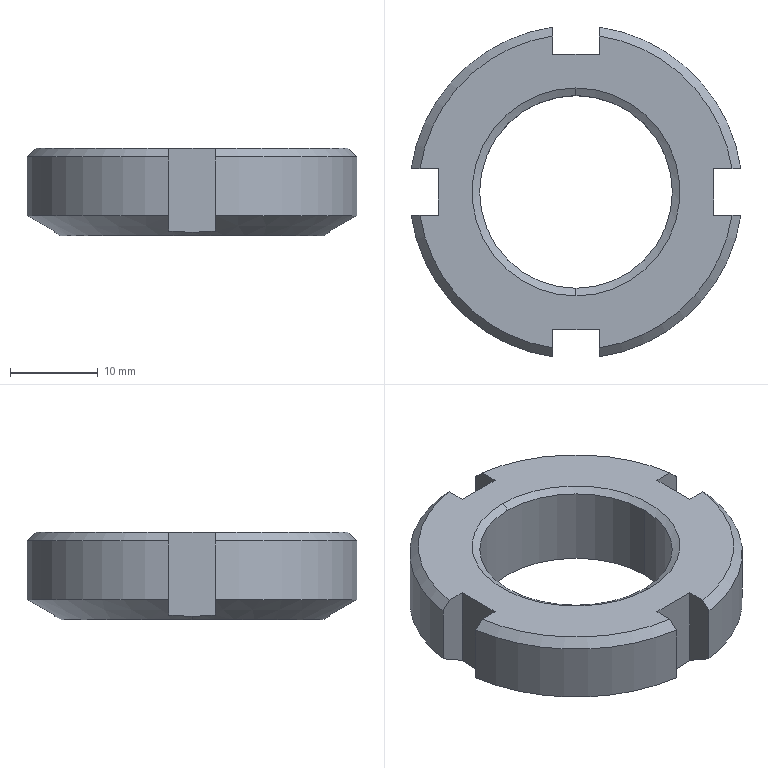Part | SolidWorks | features BaseBody 1 | 1 solid | 30 faces | box 37.629 x 37.629 x 10 mm | volume 6359 mm3 | plane 14 | cone 10 | cylinder 6 | commonest cylinder face diameters 38 x4 22 x2
STEP:
#1=CARTESIAN_POINT('',(0.,11.,9.5));
#2=VERTEX_POINT('',#1);
#3=CARTESIAN_POINT('',(-11.,0.,9.5));
#4=VERTEX_POINT('',#3);
#5=CARTESIAN_POINT('',(0.,0.,9.5));
#6=DIRECTION('',(0.,0.,1.));
#7=DIRECTION('',(1.,0.,0.));
#8=AXIS2_PLACEMENT_3D('',#5,#6,#7);
#9=CIRCLE('',#8,11.);
#10=EDGE_CURVE('',#2,#4,#9,.T.);
#11=ORIENTED_EDGE('',*,*,#10,.F.);
#12=CARTESIAN_POINT('',(0.,11.866,10.));
#13=VERTEX_POINT('',#12);
#14=CARTESIAN_POINT('',(0.,11.866,10.));
#15=DIRECTION('',(0.,0.866,0.5));
#16=VECTOR('',#15,1000.);
#17=LINE('',#14,#16);
#18=EDGE_CURVE('',#2,#13,#17,.T.);
#19=ORIENTED_EDGE('',*,*,#18,.T.);
#20=CARTESIAN_POINT('',(0.,-11.866,10.));
#21=VERTEX_POINT('',#20);
#22=CARTESIAN_POINT('',(0.,0.,10.));
#23=DIRECTION('',(0.,0.,-1.));
#24=DIRECTION('',(0.,-1.,0.));
#25=AXIS2_PLACEMENT_3D('',#22,#23,#24);
#26=CIRCLE('',#25,11.866);
#27=EDGE_CURVE('',#21,#13,#26,.T.);
#28=ORIENTED_EDGE('',*,*,#27,.F.);
#29=CARTESIAN_POINT('',(0.,-11.,9.5));
#30=VERTEX_POINT('',#29);
#31=CARTESIAN_POINT('',(0.,-11.866,10.));
#32=DIRECTION('',(0.,-0.866,0.5));
#33=VECTOR('',#32,1000.);
#34=LINE('',#31,#33);
#35=EDGE_CURVE('',#30,#21,#34,.T.);
#36=ORIENTED_EDGE('',*,*,#35,.F.);
#37=CARTESIAN_POINT('',(0.,0.,9.5));
#38=DIRECTION('',(0.,0.,1.));
#39=DIRECTION('',(1.,0.,0.));
#40=AXIS2_PLACEMENT_3D('',#37,#38,#39);
#41=CIRCLE('',#40,11.);
#42=EDGE_CURVE('',#4,#30,#41,.T.);
#43=ORIENTED_EDGE('',*,*,#42,.F.);
#44=EDGE_LOOP('',(#11,#19,#28,#36,#43));
#45=FACE_OUTER_BOUND('',#44,.T.);
#46=CARTESIAN_POINT('',(0.,0.,10.));
#47=DIRECTION('',(0.,0.,1.));
#48=DIRECTION('',(0.,-1.,0.));
#49=AXIS2_PLACEMENT_3D('',#46,#47,#48);
#50=CONICAL_SURFACE('',#49,11.866,1.047);
#51=ADVANCED_FACE('',(#45),#50,.F.);
#52=CARTESIAN_POINT('',(15.,0.,0.));
#53=VERTEX_POINT('',#52);
#54=CARTESIAN_POINT('',(-15.,0.,0.));
#55=VERTEX_POINT('',#54);
#56=CARTESIAN_POINT('',(0.,0.,0.));
#57=DIRECTION('',(0.,0.,1.));
#58=DIRECTION('',(1.,0.,0.));
#59=AXIS2_PLACEMENT_3D('',#56,#57,#58);
#60=CIRCLE('',#59,15.);
#61=EDGE_CURVE('',#53,#55,#60,.T.);
#62=ORIENTED_EDGE('',*,*,#61,.T.);
#63=CARTESIAN_POINT('',(-15.714,0.,0.4124));
#64=VERTEX_POINT('',#63);
#65=CARTESIAN_POINT('',(-19.,0.,2.309));
#66=DIRECTION('',(-0.866,0.,0.5));
#67=VECTOR('',#66,1000.);
#68=LINE('',#65,#67);
#69=EDGE_CURVE('',#55,#64,#68,.T.);
#70=ORIENTED_EDGE('',*,*,#69,.T.);
#71=CARTESIAN_POINT('',(-15.714,2.65,0.5405));
#72=VERTEX_POINT('',#71);
#73=CARTESIAN_POINT('',(-15.714,0.,0.4124));
#74=CARTESIAN_POINT('',(-15.714,0.8854,0.4124));
#75=CARTESIAN_POINT('',(-15.714,1.769,0.4559));
#76=CARTESIAN_POINT('',(-15.714,2.65,0.5405));
#77=B_SPLINE_CURVE_WITH_KNOTS('',3,(#73,#74,#75,#76),.UNSPECIFIED.,.F.,.F.,(4,4),(0.,0.002653),.UNSPECIFIED.);
#78=EDGE_CURVE('',#64,#72,#77,.T.);
#79=ORIENTED_EDGE('',*,*,#78,.T.);
#80=CARTESIAN_POINT('',(-18.814,2.65,2.309));
#81=VERTEX_POINT('',#80);
#82=CARTESIAN_POINT('',(-15.714,2.65,0.5405));
#83=CARTESIAN_POINT('',(-16.748,2.65,1.129));
#84=CARTESIAN_POINT('',(-17.781,2.65,1.719));
#85=CARTESIAN_POINT('',(-18.814,2.65,2.309));
#86=B_SPLINE_CURVE_WITH_KNOTS('',3,(#82,#83,#84,#85),.UNSPECIFIED.,.F.,.F.,(4,4),(0.,0.003569),.UNSPECIFIED.);
#87=EDGE_CURVE('',#72,#81,#86,.T.);
#88=ORIENTED_EDGE('',*,*,#87,.T.);
#89=CARTESIAN_POINT('',(-2.65,18.814,2.309));
#90=VERTEX_POINT('',#89);
#91=CARTESIAN_POINT('',(0.,0.,2.309));
#92=DIRECTION('',(0.,0.,-1.));
#93=DIRECTION('',(1.,0.,0.));
#94=AXIS2_PLACEMENT_3D('',#91,#92,#93);
#95=CIRCLE('',#94,19.);
#96=EDGE_CURVE('',#81,#90,#95,.T.);
#97=ORIENTED_EDGE('',*,*,#96,.T.);
#98=CARTESIAN_POINT('',(-2.65,15.714,0.5405));
#99=VERTEX_POINT('',#98);
#100=CARTESIAN_POINT('',(-2.65,18.814,2.309));
#101=CARTESIAN_POINT('',(-2.65,17.781,1.719));
#102=CARTESIAN_POINT('',(-2.65,16.748,1.129));
#103=CARTESIAN_POINT('',(-2.65,15.714,0.5405));
#104=B_SPLINE_CURVE_WITH_KNOTS('',3,(#100,#101,#102,#103),.UNSPECIFIED.,.F.,.F.,(4,4),(0.,0.003569),.UNSPECIFIED.);
#105=EDGE_CURVE('',#90,#99,#104,.T.);
#106=ORIENTED_EDGE('',*,*,#105,.T.);
#107=CARTESIAN_POINT('',(2.65,15.714,0.5405));
#108=VERTEX_POINT('',#107);
#109=CARTESIAN_POINT('',(-2.65,15.714,0.5405));
#110=CARTESIAN_POINT('',(-0.8833,15.714,0.3709));
#111=CARTESIAN_POINT('',(0.8833,15.714,0.3709));
#112=CARTESIAN_POINT('',(2.65,15.714,0.5405));
#113=B_SPLINE_CURVE_WITH_KNOTS('',3,(#109,#110,#111,#112),.UNSPECIFIED.,.F.,.F.,(4,4),(0.,0.0053),.UNSPECIFIED.);
#114=EDGE_CURVE('',#99,#108,#113,.T.);
#115=ORIENTED_EDGE('',*,*,#114,.T.);
#116=CARTESIAN_POINT('',(2.65,18.814,2.309));
#117=VERTEX_POINT('',#116);
#118=CARTESIAN_POINT('',(2.65,15.714,0.5405));
#119=CARTESIAN_POINT('',(2.65,16.748,1.129));
#120=CARTESIAN_POINT('',(2.65,17.781,1.719));
#121=CARTESIAN_POINT('',(2.65,18.814,2.309));
#122=B_SPLINE_CURVE_WITH_KNOTS('',3,(#118,#119,#120,#121),.UNSPECIFIED.,.F.,.F.,(4,4),(0.,0.003569),.UNSPECIFIED.);
#123=EDGE_CURVE('',#108,#117,#122,.T.);
#124=ORIENTED_EDGE('',*,*,#123,.T.);
#125=CARTESIAN_POINT('',(18.814,2.65,2.309));
#126=VERTEX_POINT('',#125);
#127=CARTESIAN_POINT('',(0.,0.,2.309));
#128=DIRECTION('',(0.,0.,-1.));
#129=DIRECTION('',(1.,0.,0.));
#130=AXIS2_PLACEMENT_3D('',#127,#128,#129);
#131=CIRCLE('',#130,19.);
#132=EDGE_CURVE('',#117,#126,#131,.T.);
#133=ORIENTED_EDGE('',*,*,#132,.T.);
#134=CARTESIAN_POINT('',(15.714,2.65,0.5405));
#135=VERTEX_POINT('',#134);
#136=CARTESIAN_POINT('',(18.814,2.65,2.309));
#137=CARTESIAN_POINT('',(17.781,2.65,1.719));
#138=CARTESIAN_POINT('',(16.748,2.65,1.129));
#139=CARTESIAN_POINT('',(15.714,2.65,0.5405));
#140=B_SPLINE_CURVE_WITH_KNOTS('',3,(#136,#137,#138,#139),.UNSPECIFIED.,.F.,.F.,(4,4),(0.,0.003569),.UNSPECIFIED.);
#141=EDGE_CURVE('',#126,#135,#140,.T.);
#142=ORIENTED_EDGE('',*,*,#141,.T.);
#143=CARTESIAN_POINT('',(15.714,0.,0.4124));
#144=VERTEX_POINT('',#143);
#145=CARTESIAN_POINT('',(15.714,2.65,0.5405));
#146=CARTESIAN_POINT('',(15.714,1.769,0.4559));
#147=CARTESIAN_POINT('',(15.714,0.8854,0.4124));
#148=CARTESIAN_POINT('',(15.714,0.,0.4124));
#149=B_SPLINE_CURVE_WITH_KNOTS('',3,(#145,#146,#147,#148),.UNSPECIFIED.,.F.,.F.,(4,4),(-0.002653,0.),.UNSPECIFIED.);
#150=EDGE_CURVE('',#135,#144,#149,.T.);
#151=ORIENTED_EDGE('',*,*,#150,.T.);
#152=CARTESIAN_POINT('',(19.,0.,2.309));
#153=DIRECTION('',(0.866,0.,0.5));
#154=VECTOR('',#153,1000.);
#155=LINE('',#152,#154);
#156=EDGE_CURVE('',#53,#144,#155,.T.);
#157=ORIENTED_EDGE('',*,*,#156,.F.);
#158=EDGE_LOOP('',(#62,#70,#79,#88,#97,#106,#115,#124,#133,#142,#151,#157));
#159=FACE_OUTER_BOUND('',#158,.T.);
#160=CARTESIAN_POINT('',(0.,0.,2.309));
#161=DIRECTION('',(0.,0.,1.));
#162=DIRECTION('',(1.,0.,0.));
#163=AXIS2_PLACEMENT_3D('',#160,#161,#162);
#164=CONICAL_SURFACE('',#163,19.,1.047);
#165=ADVANCED_FACE('',(#159),#164,.T.);
#166=ORIENTED_EDGE('',*,*,#42,.T.);
#167=CARTESIAN_POINT('',(11.,0.,9.5));
#168=VERTEX_POINT('',#167);
#169=CARTESIAN_POINT('',(0.,0.,9.5));
#170=DIRECTION('',(0.,0.,1.));
#171=DIRECTION('',(1.,0.,0.));
#172=AXIS2_PLACEMENT_3D('',#169,#170,#171);
#173=CIRCLE('',#172,11.);
#174=EDGE_CURVE('',#30,#168,#173,.T.);
#175=ORIENTED_EDGE('',*,*,#174,.T.);
#176=CARTESIAN_POINT('',(11.,0.,0.5));
#177=VERTEX_POINT('',#176);
#178=CARTESIAN_POINT('',(11.,0.,10.));
#179=DIRECTION('',(0.,0.,-1.));
#180=VECTOR('',#179,1000.);
#181=LINE('',#178,#180);
#182=EDGE_CURVE('',#168,#177,#181,.T.);
#183=ORIENTED_EDGE('',*,*,#182,.T.);
#184=CARTESIAN_POINT('',(-11.,0.,0.5));
#185=VERTEX_POINT('',#184);
#186=CARTESIAN_POINT('',(0.,0.,0.5));
#187=DIRECTION('',(0.,0.,1.));
#188=DIRECTION('',(-1.,0.,0.));
#189=AXIS2_PLACEMENT_3D('',#186,#187,#188);
#190=CIRCLE('',#189,11.);
#191=EDGE_CURVE('',#185,#177,#190,.T.);
#192=ORIENTED_EDGE('',*,*,#191,.F.);
#193=CARTESIAN_POINT('',(-11.,0.,10.));
#194=DIRECTION('',(0.,0.,-1.));
#195=VECTOR('',#194,1000.);
#196=LINE('',#193,#195);
#197=EDGE_CURVE('',#4,#185,#196,.T.);
#198=ORIENTED_EDGE('',*,*,#197,.F.);
#199=EDGE_LOOP('',(#166,#175,#183,#192,#198));
#200=FACE_OUTER_BOUND('',#199,.T.);
#201=CARTESIAN_POINT('',(0.,0.,10.));
#202=DIRECTION('',(0.,0.,-1.));
#203=DIRECTION('',(-1.,0.,0.));
#204=AXIS2_PLACEMENT_3D('',#201,#202,#203);
#205=CYLINDRICAL_SURFACE('',#204,11.);
#206=ADVANCED_FACE('',(#200),#205,.F.);
#207=ORIENTED_EDGE('',*,*,#191,.T.);
#208=CARTESIAN_POINT('',(11.866,0.,0.));
#209=VERTEX_POINT('',#208);
#210=CARTESIAN_POINT('',(11.866,0.,0.));
#211=DIRECTION('',(0.866,0.,-0.5));
#212=VECTOR('',#211,1000.);
#213=LINE('',#210,#212);
#214=EDGE_CURVE('',#177,#209,#213,.T.);
#215=ORIENTED_EDGE('',*,*,#214,.T.);
#216=CARTESIAN_POINT('',(-11.866,0.,0.));
#217=VERTEX_POINT('',#216);
#218=CARTESIAN_POINT('',(0.,0.,0.));
#219=DIRECTION('',(0.,0.,-1.));
#220=DIRECTION('',(-1.,0.,0.));
#221=AXIS2_PLACEMENT_3D('',#218,#219,#220);
#222=CIRCLE('',#221,11.866);
#223=EDGE_CURVE('',#209,#217,#222,.T.);
#224=ORIENTED_EDGE('',*,*,#223,.T.);
#225=CARTESIAN_POINT('',(-11.866,0.,0.));
#226=DIRECTION('',(-0.866,0.,-0.5));
#227=VECTOR('',#226,1000.);
#228=LINE('',#225,#227);
#229=EDGE_CURVE('',#185,#217,#228,.T.);
#230=ORIENTED_EDGE('',*,*,#229,.F.);
#231=EDGE_LOOP('',(#207,#215,#224,#230));
#232=FACE_OUTER_BOUND('',#231,.T.);
#233=CARTESIAN_POINT('',(0.,0.,0.));
#234=DIRECTION('',(0.,0.,-1.));
#235=DIRECTION('',(-1.,0.,0.));
#236=AXIS2_PLACEMENT_3D('',#233,#234,#235);
#237=CONICAL_SURFACE('',#236,11.866,1.047);
#238=ADVANCED_FACE('',(#232),#237,.F.);
#239=CARTESIAN_POINT('',(17.804,-2.65,10.));
#240=VERTEX_POINT('',#239);
#241=CARTESIAN_POINT('',(15.714,-2.65,10.));
#242=VERTEX_POINT('',#241);
#243=CARTESIAN_POINT('',(0.,-2.65,10.));
#244=DIRECTION('',(-1.,0.,0.));
#245=VECTOR('',#244,1000.);
#246=LINE('',#243,#245);
#247=EDGE_CURVE('',#240,#242,#246,.T.);
#248=ORIENTED_EDGE('',*,*,#247,.T.);
#249=CARTESIAN_POINT('',(15.714,2.65,10.));
#250=VERTEX_POINT('',#249);
#251=CARTESIAN_POINT('',(15.714,0.,10.));
#252=DIRECTION('',(0.,1.,0.));
#253=VECTOR('',#252,1000.);
#254=LINE('',#251,#253);
#255=EDGE_CURVE('',#242,#250,#254,.T.);
#256=ORIENTED_EDGE('',*,*,#255,.T.);
#257=CARTESIAN_POINT('',(17.804,2.65,10.));
#258=VERTEX_POINT('',#257);
#259=CARTESIAN_POINT('',(0.,2.65,10.));
#260=DIRECTION('',(1.,0.,0.));
#261=VECTOR('',#260,1000.);
#262=LINE('',#259,#261);
#263=EDGE_CURVE('',#250,#258,#262,.T.);
#264=ORIENTED_EDGE('',*,*,#263,.T.);
#265=CARTESIAN_POINT('',(2.65,17.804,10.));
#266=VERTEX_POINT('',#265);
#267=CARTESIAN_POINT('',(0.,0.,10.));
#268=DIRECTION('',(0.,0.,1.));
#269=DIRECTION('',(-1.,0.,0.));
#270=AXIS2_PLACEMENT_3D('',#267,#268,#269);
#271=CIRCLE('',#270,18.);
#272=EDGE_CURVE('',#258,#266,#271,.T.);
#273=ORIENTED_EDGE('',*,*,#272,.T.);
#274=CARTESIAN_POINT('',(2.65,15.714,10.));
#275=VERTEX_POINT('',#274);
#276=CARTESIAN_POINT('',(2.65,0.,10.));
#277=DIRECTION('',(0.,-1.,0.));
#278=VECTOR('',#277,1000.);
#279=LINE('',#276,#278);
#280=EDGE_CURVE('',#266,#275,#279,.T.);
#281=ORIENTED_EDGE('',*,*,#280,.T.);
#282=CARTESIAN_POINT('',(-2.65,15.714,10.));
#283=VERTEX_POINT('',#282);
#284=CARTESIAN_POINT('',(0.,15.714,10.));
#285=DIRECTION('',(-1.,0.,0.));
#286=VECTOR('',#285,1000.);
#287=LINE('',#284,#286);
#288=EDGE_CURVE('',#275,#283,#287,.T.);
#289=ORIENTED_EDGE('',*,*,#288,.T.);
#290=CARTESIAN_POINT('',(-2.65,17.804,10.));
#291=VERTEX_POINT('',#290);
#292=CARTESIAN_POINT('',(-2.65,0.,10.));
#293=DIRECTION('',(0.,1.,0.));
#294=VECTOR('',#293,1000.);
#295=LINE('',#292,#294);
#296=EDGE_CURVE('',#283,#291,#295,.T.);
#297=ORIENTED_EDGE('',*,*,#296,.T.);
#298=CARTESIAN_POINT('',(-17.804,2.65,10.));
#299=VERTEX_POINT('',#298);
#300=CARTESIAN_POINT('',(0.,0.,10.));
#301=DIRECTION('',(0.,0.,1.));
#302=DIRECTION('',(0.,1.,0.));
#303=AXIS2_PLACEMENT_3D('',#300,#301,#302);
#304=CIRCLE('',#303,18.);
#305=EDGE_CURVE('',#291,#299,#304,.T.);
#306=ORIENTED_EDGE('',*,*,#305,.T.);
#307=CARTESIAN_POINT('',(-15.714,2.65,10.));
#308=VERTEX_POINT('',#307);
#309=CARTESIAN_POINT('',(0.,2.65,10.));
#310=DIRECTION('',(1.,0.,0.));
#311=VECTOR('',#310,1000.);
#312=LINE('',#309,#311);
#313=EDGE_CURVE('',#299,#308,#312,.T.);
#314=ORIENTED_EDGE('',*,*,#313,.T.);
#315=CARTESIAN_POINT('',(-15.714,-2.65,10.));
#316=VERTEX_POINT('',#315);
#317=CARTESIAN_POINT('',(-15.714,0.,10.));
#318=DIRECTION('',(0.,-1.,0.));
#319=VECTOR('',#318,1000.);
#320=LINE('',#317,#319);
#321=EDGE_CURVE('',#308,#316,#320,.T.);
#322=ORIENTED_EDGE('',*,*,#321,.T.);
#323=CARTESIAN_POINT('',(-17.804,-2.65,10.));
#324=VERTEX_POINT('',#323);
#325=CARTESIAN_POINT('',(0.,-2.65,10.));
#326=DIRECTION('',(-1.,0.,0.));
#327=VECTOR('',#326,1000.);
#328=LINE('',#325,#327);
#329=EDGE_CURVE('',#316,#324,#328,.T.);
#330=ORIENTED_EDGE('',*,*,#329,.T.);
#331=CARTESIAN_POINT('',(-2.65,-17.804,10.));
#332=VERTEX_POINT('',#331);
#333=CARTESIAN_POINT('',(0.,0.,10.));
#334=DIRECTION('',(0.,0.,1.));
#335=DIRECTION('',(-1.,0.,0.));
#336=AXIS2_PLACEMENT_3D('',#333,#334,#335);
#337=CIRCLE('',#336,18.);
#338=EDGE_CURVE('',#324,#332,#337,.T.);
#339=ORIENTED_EDGE('',*,*,#338,.T.);
#340=CARTESIAN_POINT('',(-2.65,-15.714,10.));
#341=VERTEX_POINT('',#340);
#342=CARTESIAN_POINT('',(-2.65,0.,10.));
#343=DIRECTION('',(0.,1.,0.));
#344=VECTOR('',#343,1000.);
#345=LINE('',#342,#344);
#346=EDGE_CURVE('',#332,#341,#345,.T.);
#347=ORIENTED_EDGE('',*,*,#346,.T.);
#348=CARTESIAN_POINT('',(2.65,-15.714,10.));
#349=VERTEX_POINT('',#348);
#350=CARTESIAN_POINT('',(0.,-15.714,10.));
#351=DIRECTION('',(1.,0.,0.));
#352=VECTOR('',#351,1000.);
#353=LINE('',#350,#352);
#354=EDGE_CURVE('',#341,#349,#353,.T.);
#355=ORIENTED_EDGE('',*,*,#354,.T.);
#356=CARTESIAN_POINT('',(2.65,-17.804,10.));
#357=VERTEX_POINT('',#356);
#358=CARTESIAN_POINT('',(2.65,0.,10.));
#359=DIRECTION('',(0.,-1.,0.));
#360=VECTOR('',#359,1000.);
#361=LINE('',#358,#360);
#362=EDGE_CURVE('',#349,#357,#361,.T.);
#363=ORIENTED_EDGE('',*,*,#362,.T.);
#364=CARTESIAN_POINT('',(0.,0.,10.));
#365=DIRECTION('',(0.,0.,1.));
#366=DIRECTION('',(-1.,0.,0.));
#367=AXIS2_PLACEMENT_3D('',#364,#365,#366);
#368=CIRCLE('',#367,18.);
#369=EDGE_CURVE('',#357,#240,#368,.T.);
#370=ORIENTED_EDGE('',*,*,#369,.T.);
#371=EDGE_LOOP('',(#248,#256,#264,#273,#281,#289,#297,#306,#314,#322,#330,#339,#347,#355,#363,#370));
#372=FACE_OUTER_BOUND('',#371,.T.);
#373=ORIENTED_EDGE('',*,*,#27,.T.);
#374=CARTESIAN_POINT('',(0.,0.,10.));
#375=DIRECTION('',(0.,0.,-1.));
#376=DIRECTION('',(0.,-1.,0.));
#377=AXIS2_PLACEMENT_3D('',#374,#375,#376);
#378=CIRCLE('',#377,11.866);
#379=EDGE_CURVE('',#13,#21,#378,.T.);
#380=ORIENTED_EDGE('',*,*,#379,.T.);
#381=EDGE_LOOP('',(#373,#380));
#382=FACE_BOUND('',#381,.T.);
#383=CARTESIAN_POINT('',(0.,0.,10.));
#384=DIRECTION('',(0.,0.,1.));
#385=DIRECTION('',(1.,0.,0.));
#386=AXIS2_PLACEMENT_3D('',#383,#384,#385);
#387=PLANE('',#386);
#388=ADVANCED_FACE('',(#372,#382),#387,.T.);
#389=ORIENTED_EDGE('',*,*,#150,.F.);
#390=CARTESIAN_POINT('',(15.714,2.65,0.));
#391=DIRECTION('',(0.,0.,-1.));
#392=VECTOR('',#391,1000.);
#393=LINE('',#390,#392);
#394=EDGE_CURVE('',#250,#135,#393,.T.);
#395=ORIENTED_EDGE('',*,*,#394,.F.);
#396=ORIENTED_EDGE('',*,*,#255,.F.);
#397=CARTESIAN_POINT('',(15.714,-2.65,0.5405));
#398=VERTEX_POINT('',#397);
#399=CARTESIAN_POINT('',(15.714,-2.65,0.));
#400=DIRECTION('',(0.,0.,1.));
#401=VECTOR('',#400,1000.);
#402=LINE('',#399,#401);
#403=EDGE_CURVE('',#398,#242,#402,.T.);
#404=ORIENTED_EDGE('',*,*,#403,.F.);
#405=CARTESIAN_POINT('',(15.714,0.,0.4124));
#406=CARTESIAN_POINT('',(15.714,-0.8854,0.4124));
#407=CARTESIAN_POINT('',(15.714,-1.769,0.4559));
#408=CARTESIAN_POINT('',(15.714,-2.65,0.5405));
#409=B_SPLINE_CURVE_WITH_KNOTS('',3,(#405,#406,#407,#408),.UNSPECIFIED.,.F.,.F.,(4,4),(0.,0.002653),.UNSPECIFIED.);
#410=EDGE_CURVE('',#144,#398,#409,.T.);
#411=ORIENTED_EDGE('',*,*,#410,.F.);
#412=EDGE_LOOP('',(#389,#395,#396,#404,#411));
#413=FACE_OUTER_BOUND('',#412,.T.);
#414=CARTESIAN_POINT('',(15.714,-2.65,0.));
#415=DIRECTION('',(-1.,0.,0.));
#416=DIRECTION('',(0.,-1.,0.));
#417=AXIS2_PLACEMENT_3D('',#414,#415,#416);
#418=PLANE('',#417);
#419=ADVANCED_FACE('',(#413),#418,.F.);
#420=CARTESIAN_POINT('',(18.814,-2.65,2.309));
#421=VERTEX_POINT('',#420);
#422=CARTESIAN_POINT('',(18.814,-2.65,9.));
#423=VERTEX_POINT('',#422);
#424=CARTESIAN_POINT('',(18.814,-2.65,0.));
#425=DIRECTION('',(0.,0.,1.));
#426=VECTOR('',#425,1000.);
#427=LINE('',#424,#426);
#428=EDGE_CURVE('',#421,#423,#427,.T.);
#429=ORIENTED_EDGE('',*,*,#428,.F.);
#430=CARTESIAN_POINT('',(15.714,-2.65,0.5405));
#431=CARTESIAN_POINT('',(16.748,-2.65,1.129));
#432=CARTESIAN_POINT('',(17.781,-2.65,1.719));
#433=CARTESIAN_POINT('',(18.814,-2.65,2.309));
#434=B_SPLINE_CURVE_WITH_KNOTS('',3,(#430,#431,#432,#433),.UNSPECIFIED.,.F.,.F.,(4,4),(0.,0.003569),.UNSPECIFIED.);
#435=EDGE_CURVE('',#398,#421,#434,.T.);
#436=ORIENTED_EDGE('',*,*,#435,.F.);
#437=ORIENTED_EDGE('',*,*,#403,.T.);
#438=ORIENTED_EDGE('',*,*,#247,.F.);
#439=CARTESIAN_POINT('',(18.814,-2.65,9.));
#440=CARTESIAN_POINT('',(18.478,-2.65,9.333));
#441=CARTESIAN_POINT('',(18.141,-2.65,9.667));
#442=CARTESIAN_POINT('',(17.804,-2.65,10.));
#443=B_SPLINE_CURVE_WITH_KNOTS('',3,(#439,#440,#441,#442),.UNSPECIFIED.,.F.,.F.,(4,4),(0.,0.001422),.UNSPECIFIED.);
#444=EDGE_CURVE('',#423,#240,#443,.T.);
#445=ORIENTED_EDGE('',*,*,#444,.F.);
#446=EDGE_LOOP('',(#429,#436,#437,#438,#445));
#447=FACE_OUTER_BOUND('',#446,.T.);
#448=CARTESIAN_POINT('',(15.714,-2.65,0.));
#449=DIRECTION('',(0.,-1.,0.));
#450=DIRECTION('',(1.,0.,0.));
#451=AXIS2_PLACEMENT_3D('',#448,#449,#450);
#452=PLANE('',#451);
#453=ADVANCED_FACE('',(#447),#452,.F.);
#454=CARTESIAN_POINT('',(2.65,-18.814,9.));
#455=VERTEX_POINT('',#454);
#456=CARTESIAN_POINT('',(2.65,-17.804,10.));
#457=CARTESIAN_POINT('',(2.65,-18.141,9.667));
#458=CARTESIAN_POINT('',(2.65,-18.478,9.333));
#459=CARTESIAN_POINT('',(2.65,-18.814,9.));
#460=B_SPLINE_CURVE_WITH_KNOTS('',3,(#456,#457,#458,#459),.UNSPECIFIED.,.F.,.F.,(4,4),(0.,0.001422),.UNSPECIFIED.);
#461=EDGE_CURVE('',#357,#455,#460,.T.);
#462=ORIENTED_EDGE('',*,*,#461,.T.);
#463=CARTESIAN_POINT('',(0.,0.,9.));
#464=DIRECTION('',(0.,0.,1.));
#465=DIRECTION('',(-1.,0.,0.));
#466=AXIS2_PLACEMENT_3D('',#463,#464,#465);
#467=CIRCLE('',#466,19.);
#468=EDGE_CURVE('',#455,#423,#467,.T.);
#469=ORIENTED_EDGE('',*,*,#468,.T.);
#470=ORIENTED_EDGE('',*,*,#444,.T.);
#471=ORIENTED_EDGE('',*,*,#369,.F.);
#472=EDGE_LOOP('',(#462,#469,#470,#471));
#473=FACE_OUTER_BOUND('',#472,.T.);
#474=CARTESIAN_POINT('',(0.,0.,9.));
#475=DIRECTION('',(0.,0.,-1.));
#476=DIRECTION('',(-1.,0.,0.));
#477=AXIS2_PLACEMENT_3D('',#474,#475,#476);
#478=CONICAL_SURFACE('',#477,19.,0.7854);
#479=ADVANCED_FACE('',(#473),#478,.T.);
#480=ORIENTED_EDGE('',*,*,#362,.F.);
#481=CARTESIAN_POINT('',(2.65,-15.714,0.5405));
#482=VERTEX_POINT('',#481);
#483=CARTESIAN_POINT('',(2.65,-15.714,0.));
#484=DIRECTION('',(0.,0.,1.));
#485=VECTOR('',#484,1000.);
#486=LINE('',#483,#485);
#487=EDGE_CURVE('',#482,#349,#486,.T.);
#488=ORIENTED_EDGE('',*,*,#487,.F.);
#489=CARTESIAN_POINT('',(2.65,-18.814,2.309));
#490=VERTEX_POINT('',#489);
#491=CARTESIAN_POINT('',(2.65,-18.814,2.309));
#492=CARTESIAN_POINT('',(2.65,-17.781,1.719));
#493=CARTESIAN_POINT('',(2.65,-16.748,1.129));
#494=CARTESIAN_POINT('',(2.65,-15.714,0.5405));
#495=B_SPLINE_CURVE_WITH_KNOTS('',3,(#491,#492,#493,#494),.UNSPECIFIED.,.F.,.F.,(4,4),(0.,0.003569),.UNSPECIFIED.);
#496=EDGE_CURVE('',#490,#482,#495,.T.);
#497=ORIENTED_EDGE('',*,*,#496,.F.);
#498=CARTESIAN_POINT('',(2.65,-18.814,0.));
#499=DIRECTION('',(0.,0.,-1.));
#500=VECTOR('',#499,1000.);
#501=LINE('',#498,#500);
#502=EDGE_CURVE('',#455,#490,#501,.T.);
#503=ORIENTED_EDGE('',*,*,#502,.F.);
#504=ORIENTED_EDGE('',*,*,#461,.F.);
#505=EDGE_LOOP('',(#480,#488,#497,#503,#504));
#506=FACE_OUTER_BOUND('',#505,.T.);
#507=CARTESIAN_POINT('',(2.65,-15.714,0.));
#508=DIRECTION('',(1.,0.,0.));
#509=DIRECTION('',(0.,1.,0.));
#510=AXIS2_PLACEMENT_3D('',#507,#508,#509);
#511=PLANE('',#510);
#512=ADVANCED_FACE('',(#506),#511,.F.);
#513=ORIENTED_EDGE('',*,*,#487,.T.);
#514=ORIENTED_EDGE('',*,*,#354,.F.);
#515=CARTESIAN_POINT('',(-2.65,-15.714,0.5405));
#516=VERTEX_POINT('',#515);
#517=CARTESIAN_POINT('',(-2.65,-15.714,0.));
#518=DIRECTION('',(0.,0.,1.));
#519=VECTOR('',#518,1000.);
#520=LINE('',#517,#519);
#521=EDGE_CURVE('',#516,#341,#520,.T.);
#522=ORIENTED_EDGE('',*,*,#521,.F.);
#523=CARTESIAN_POINT('',(2.65,-15.714,0.5405));
#524=CARTESIAN_POINT('',(0.8833,-15.714,0.3709));
#525=CARTESIAN_POINT('',(-0.8833,-15.714,0.3709));
#526=CARTESIAN_POINT('',(-2.65,-15.714,0.5405));
#527=B_SPLINE_CURVE_WITH_KNOTS('',3,(#523,#524,#525,#526),.UNSPECIFIED.,.F.,.F.,(4,4),(0.,0.0053),.UNSPECIFIED.);
#528=EDGE_CURVE('',#482,#516,#527,.T.);
#529=ORIENTED_EDGE('',*,*,#528,.F.);
#530=EDGE_LOOP('',(#513,#514,#522,#529));
#531=FACE_OUTER_BOUND('',#530,.T.);
#532=CARTESIAN_POINT('',(-2.65,-15.714,0.));
#533=DIRECTION('',(0.,1.,0.));
#534=DIRECTION('',(0.,0.,1.));
#535=AXIS2_PLACEMENT_3D('',#532,#533,#534);
#536=PLANE('',#535);
#537=ADVANCED_FACE('',(#531),#536,.F.);
#538=CARTESIAN_POINT('',(-2.65,-18.814,2.309));
#539=VERTEX_POINT('',#538);
#540=CARTESIAN_POINT('',(-2.65,-18.814,9.));
#541=VERTEX_POINT('',#540);
#542=CARTESIAN_POINT('',(-2.65,-18.814,0.));
#543=DIRECTION('',(0.,0.,1.));
#544=VECTOR('',#543,1000.);
#545=LINE('',#542,#544);
#546=EDGE_CURVE('',#539,#541,#545,.T.);
#547=ORIENTED_EDGE('',*,*,#546,.F.);
#548=CARTESIAN_POINT('',(-2.65,-15.714,0.5405));
#549=CARTESIAN_POINT('',(-2.65,-16.748,1.129));
#550=CARTESIAN_POINT('',(-2.65,-17.781,1.719));
#551=CARTESIAN_POINT('',(-2.65,-18.814,2.309));
#552=B_SPLINE_CURVE_WITH_KNOTS('',3,(#548,#549,#550,#551),.UNSPECIFIED.,.F.,.F.,(4,4),(0.,0.003569),.UNSPECIFIED.);
#553=EDGE_CURVE('',#516,#539,#552,.T.);
#554=ORIENTED_EDGE('',*,*,#553,.F.);
#555=ORIENTED_EDGE('',*,*,#521,.T.);
#556=ORIENTED_EDGE('',*,*,#346,.F.);
#557=CARTESIAN_POINT('',(-2.65,-18.814,9.));
#558=CARTESIAN_POINT('',(-2.65,-18.478,9.333));
#559=CARTESIAN_POINT('',(-2.65,-18.141,9.667));
#560=CARTESIAN_POINT('',(-2.65,-17.804,10.));
#561=B_SPLINE_CURVE_WITH_KNOTS('',3,(#557,#558,#559,#560),.UNSPECIFIED.,.F.,.F.,(4,4),(0.,0.001422),.UNSPECIFIED.);
#562=EDGE_CURVE('',#541,#332,#561,.T.);
#563=ORIENTED_EDGE('',*,*,#562,.F.);
#564=EDGE_LOOP('',(#547,#554,#555,#556,#563));
#565=FACE_OUTER_BOUND('',#564,.T.);
#566=CARTESIAN_POINT('',(-2.65,-15.714,0.));
#567=DIRECTION('',(-1.,0.,0.));
#568=DIRECTION('',(0.,-1.,0.));
#569=AXIS2_PLACEMENT_3D('',#566,#567,#568);
#570=PLANE('',#569);
#571=ADVANCED_FACE('',(#565),#570,.F.);
#572=ORIENTED_EDGE('',*,*,#562,.T.);
#573=ORIENTED_EDGE('',*,*,#338,.F.);
#574=CARTESIAN_POINT('',(-18.814,-2.65,9.));
#575=VERTEX_POINT('',#574);
#576=CARTESIAN_POINT('',(-17.804,-2.65,10.));
#577=CARTESIAN_POINT('',(-18.141,-2.65,9.667));
#578=CARTESIAN_POINT('',(-18.478,-2.65,9.333));
#579=CARTESIAN_POINT('',(-18.814,-2.65,9.));
#580=B_SPLINE_CURVE_WITH_KNOTS('',3,(#576,#577,#578,#579),.UNSPECIFIED.,.F.,.F.,(4,4),(0.,0.001422),.UNSPECIFIED.);
#581=EDGE_CURVE('',#324,#575,#580,.T.);
#582=ORIENTED_EDGE('',*,*,#581,.T.);
#583=CARTESIAN_POINT('',(0.,0.,9.));
#584=DIRECTION('',(0.,0.,1.));
#585=DIRECTION('',(-1.,0.,0.));
#586=AXIS2_PLACEMENT_3D('',#583,#584,#585);
#587=CIRCLE('',#586,19.);
#588=EDGE_CURVE('',#575,#541,#587,.T.);
#589=ORIENTED_EDGE('',*,*,#588,.T.);
#590=EDGE_LOOP('',(#572,#573,#582,#589));
#591=FACE_OUTER_BOUND('',#590,.T.);
#592=CARTESIAN_POINT('',(0.,0.,9.));
#593=DIRECTION('',(0.,0.,-1.));
#594=DIRECTION('',(-1.,0.,0.));
#595=AXIS2_PLACEMENT_3D('',#592,#593,#594);
#596=CONICAL_SURFACE('',#595,19.,0.7854);
#597=ADVANCED_FACE('',(#591),#596,.T.);
#598=ORIENTED_EDGE('',*,*,#329,.F.);
#599=CARTESIAN_POINT('',(-15.714,-2.65,0.5405));
#600=VERTEX_POINT('',#599);
#601=CARTESIAN_POINT('',(-15.714,-2.65,0.));
#602=DIRECTION('',(0.,0.,1.));
#603=VECTOR('',#602,1000.);
#604=LINE('',#601,#603);
#605=EDGE_CURVE('',#600,#316,#604,.T.);
#606=ORIENTED_EDGE('',*,*,#605,.F.);
#607=CARTESIAN_POINT('',(-18.814,-2.65,2.309));
#608=VERTEX_POINT('',#607);
#609=CARTESIAN_POINT('',(-18.814,-2.65,2.309));
#610=CARTESIAN_POINT('',(-17.781,-2.65,1.719));
#611=CARTESIAN_POINT('',(-16.748,-2.65,1.129));
#612=CARTESIAN_POINT('',(-15.714,-2.65,0.5405));
#613=B_SPLINE_CURVE_WITH_KNOTS('',3,(#609,#610,#611,#612),.UNSPECIFIED.,.F.,.F.,(4,4),(0.,0.003569),.UNSPECIFIED.);
#614=EDGE_CURVE('',#608,#600,#613,.T.);
#615=ORIENTED_EDGE('',*,*,#614,.F.);
#616=CARTESIAN_POINT('',(-18.814,-2.65,0.));
#617=DIRECTION('',(0.,0.,-1.));
#618=VECTOR('',#617,1000.);
#619=LINE('',#616,#618);
#620=EDGE_CURVE('',#575,#608,#619,.T.);
#621=ORIENTED_EDGE('',*,*,#620,.F.);
#622=ORIENTED_EDGE('',*,*,#581,.F.);
#623=EDGE_LOOP('',(#598,#606,#615,#621,#622));
#624=FACE_OUTER_BOUND('',#623,.T.);
#625=CARTESIAN_POINT('',(-15.714,-2.65,0.));
#626=DIRECTION('',(0.,-1.,0.));
#627=DIRECTION('',(1.,0.,0.));
#628=AXIS2_PLACEMENT_3D('',#625,#626,#627);
#629=PLANE('',#628);
#630=ADVANCED_FACE('',(#624),#629,.F.);
#631=CARTESIAN_POINT('',(-15.714,-2.65,0.5405));
#632=CARTESIAN_POINT('',(-15.714,-1.769,0.4559));
#633=CARTESIAN_POINT('',(-15.714,-0.8854,0.4124));
#634=CARTESIAN_POINT('',(-15.714,0.,0.4124));
#635=B_SPLINE_CURVE_WITH_KNOTS('',3,(#631,#632,#633,#634),.UNSPECIFIED.,.F.,.F.,(4,4),(-0.002653,0.),.UNSPECIFIED.);
#636=EDGE_CURVE('',#600,#64,#635,.T.);
#637=ORIENTED_EDGE('',*,*,#636,.F.);
#638=ORIENTED_EDGE('',*,*,#605,.T.);
#639=ORIENTED_EDGE('',*,*,#321,.F.);
#640=CARTESIAN_POINT('',(-15.714,2.65,0.));
#641=DIRECTION('',(0.,0.,1.));
#642=VECTOR('',#641,1000.);
#643=LINE('',#640,#642);
#644=EDGE_CURVE('',#72,#308,#643,.T.);
#645=ORIENTED_EDGE('',*,*,#644,.F.);
#646=ORIENTED_EDGE('',*,*,#78,.F.);
#647=EDGE_LOOP('',(#637,#638,#639,#645,#646));
#648=FACE_OUTER_BOUND('',#647,.T.);
#649=CARTESIAN_POINT('',(-15.714,2.65,0.));
#650=DIRECTION('',(1.,0.,0.));
#651=DIRECTION('',(0.,1.,0.));
#652=AXIS2_PLACEMENT_3D('',#649,#650,#651);
#653=PLANE('',#652);
#654=ADVANCED_FACE('',(#648),#653,.F.);
#655=CARTESIAN_POINT('',(-18.814,2.65,9.));
#656=VERTEX_POINT('',#655);
#657=CARTESIAN_POINT('',(-18.814,2.65,0.));
#658=DIRECTION('',(0.,0.,1.));
#659=VECTOR('',#658,1000.);
#660=LINE('',#657,#659);
#661=EDGE_CURVE('',#81,#656,#660,.T.);
#662=ORIENTED_EDGE('',*,*,#661,.F.);
#663=ORIENTED_EDGE('',*,*,#87,.F.);
#664=ORIENTED_EDGE('',*,*,#644,.T.);
#665=ORIENTED_EDGE('',*,*,#313,.F.);
#666=CARTESIAN_POINT('',(-18.814,2.65,9.));
#667=CARTESIAN_POINT('',(-18.478,2.65,9.333));
#668=CARTESIAN_POINT('',(-18.141,2.65,9.667));
#669=CARTESIAN_POINT('',(-17.804,2.65,10.));
#670=B_SPLINE_CURVE_WITH_KNOTS('',3,(#666,#667,#668,#669),.UNSPECIFIED.,.F.,.F.,(4,4),(0.,0.001422),.UNSPECIFIED.);
#671=EDGE_CURVE('',#656,#299,#670,.T.);
#672=ORIENTED_EDGE('',*,*,#671,.F.);
#673=EDGE_LOOP('',(#662,#663,#664,#665,#672));
#674=FACE_OUTER_BOUND('',#673,.T.);
#675=CARTESIAN_POINT('',(-15.714,2.65,0.));
#676=DIRECTION('',(0.,1.,0.));
#677=DIRECTION('',(-1.,0.,0.));
#678=AXIS2_PLACEMENT_3D('',#675,#676,#677);
#679=PLANE('',#678);
#680=ADVANCED_FACE('',(#674),#679,.F.);
#681=ORIENTED_EDGE('',*,*,#671,.T.);
#682=ORIENTED_EDGE('',*,*,#305,.F.);
#683=CARTESIAN_POINT('',(-2.65,18.814,9.));
#684=VERTEX_POINT('',#683);
#685=CARTESIAN_POINT('',(-2.65,17.804,10.));
#686=CARTESIAN_POINT('',(-2.65,18.141,9.667));
#687=CARTESIAN_POINT('',(-2.65,18.478,9.333));
#688=CARTESIAN_POINT('',(-2.65,18.814,9.));
#689=B_SPLINE_CURVE_WITH_KNOTS('',3,(#685,#686,#687,#688),.UNSPECIFIED.,.F.,.F.,(4,4),(0.,0.001422),.UNSPECIFIED.);
#690=EDGE_CURVE('',#291,#684,#689,.T.);
#691=ORIENTED_EDGE('',*,*,#690,.T.);
#692=CARTESIAN_POINT('',(0.,0.,9.));
#693=DIRECTION('',(0.,0.,1.));
#694=DIRECTION('',(-1.,0.,0.));
#695=AXIS2_PLACEMENT_3D('',#692,#693,#694);
#696=CIRCLE('',#695,19.);
#697=EDGE_CURVE('',#684,#656,#696,.T.);
#698=ORIENTED_EDGE('',*,*,#697,.T.);
#699=EDGE_LOOP('',(#681,#682,#691,#698));
#700=FACE_OUTER_BOUND('',#699,.T.);
#701=CARTESIAN_POINT('',(0.,0.,9.));
#702=DIRECTION('',(0.,0.,-1.));
#703=DIRECTION('',(0.,1.,0.));
#704=AXIS2_PLACEMENT_3D('',#701,#702,#703);
#705=CONICAL_SURFACE('',#704,19.,0.7854);
#706=ADVANCED_FACE('',(#700),#705,.T.);
#707=ORIENTED_EDGE('',*,*,#296,.F.);
#708=CARTESIAN_POINT('',(-2.65,15.714,0.));
#709=DIRECTION('',(0.,0.,1.));
#710=VECTOR('',#709,1000.);
#711=LINE('',#708,#710);
#712=EDGE_CURVE('',#99,#283,#711,.T.);
#713=ORIENTED_EDGE('',*,*,#712,.F.);
#714=ORIENTED_EDGE('',*,*,#105,.F.);
#715=CARTESIAN_POINT('',(-2.65,18.814,0.));
#716=DIRECTION('',(0.,0.,-1.));
#717=VECTOR('',#716,1000.);
#718=LINE('',#715,#717);
#719=EDGE_CURVE('',#684,#90,#718,.T.);
#720=ORIENTED_EDGE('',*,*,#719,.F.);
#721=ORIENTED_EDGE('',*,*,#690,.F.);
#722=EDGE_LOOP('',(#707,#713,#714,#720,#721));
#723=FACE_OUTER_BOUND('',#722,.T.);
#724=CARTESIAN_POINT('',(-2.65,15.714,0.));
#725=DIRECTION('',(-1.,0.,0.));
#726=DIRECTION('',(0.,-1.,0.));
#727=AXIS2_PLACEMENT_3D('',#724,#725,#726);
#728=PLANE('',#727);
#729=ADVANCED_FACE('',(#723),#728,.F.);
#730=ORIENTED_EDGE('',*,*,#712,.T.);
#731=ORIENTED_EDGE('',*,*,#288,.F.);
#732=CARTESIAN_POINT('',(2.65,15.714,0.));
#733=DIRECTION('',(0.,0.,1.));
#734=VECTOR('',#733,1000.);
#735=LINE('',#732,#734);
#736=EDGE_CURVE('',#108,#275,#735,.T.);
#737=ORIENTED_EDGE('',*,*,#736,.F.);
#738=ORIENTED_EDGE('',*,*,#114,.F.);
#739=EDGE_LOOP('',(#730,#731,#737,#738));
#740=FACE_OUTER_BOUND('',#739,.T.);
#741=CARTESIAN_POINT('',(2.65,15.714,0.));
#742=DIRECTION('',(0.,-1.,0.));
#743=DIRECTION('',(1.,0.,0.));
#744=AXIS2_PLACEMENT_3D('',#741,#742,#743);
#745=PLANE('',#744);
#746=ADVANCED_FACE('',(#740),#745,.F.);
#747=CARTESIAN_POINT('',(2.65,18.814,9.));
#748=VERTEX_POINT('',#747);
#749=CARTESIAN_POINT('',(2.65,18.814,0.));
#750=DIRECTION('',(0.,0.,1.));
#751=VECTOR('',#750,1000.);
#752=LINE('',#749,#751);
#753=EDGE_CURVE('',#117,#748,#752,.T.);
#754=ORIENTED_EDGE('',*,*,#753,.F.);
#755=ORIENTED_EDGE('',*,*,#123,.F.);
#756=ORIENTED_EDGE('',*,*,#736,.T.);
#757=ORIENTED_EDGE('',*,*,#280,.F.);
#758=CARTESIAN_POINT('',(2.65,18.814,9.));
#759=CARTESIAN_POINT('',(2.65,18.478,9.333));
#760=CARTESIAN_POINT('',(2.65,18.141,9.667));
#761=CARTESIAN_POINT('',(2.65,17.804,10.));
#762=B_SPLINE_CURVE_WITH_KNOTS('',3,(#758,#759,#760,#761),.UNSPECIFIED.,.F.,.F.,(4,4),(0.,0.001422),.UNSPECIFIED.);
#763=EDGE_CURVE('',#748,#266,#762,.T.);
#764=ORIENTED_EDGE('',*,*,#763,.F.);
#765=EDGE_LOOP('',(#754,#755,#756,#757,#764));
#766=FACE_OUTER_BOUND('',#765,.T.);
#767=CARTESIAN_POINT('',(2.65,15.714,0.));
#768=DIRECTION('',(1.,0.,0.));
#769=DIRECTION('',(0.,1.,0.));
#770=AXIS2_PLACEMENT_3D('',#767,#768,#769);
#771=PLANE('',#770);
#772=ADVANCED_FACE('',(#766),#771,.F.);
#773=ORIENTED_EDGE('',*,*,#763,.T.);
#774=ORIENTED_EDGE('',*,*,#272,.F.);
#775=CARTESIAN_POINT('',(18.814,2.65,9.));
#776=VERTEX_POINT('',#775);
#777=CARTESIAN_POINT('',(17.804,2.65,10.));
#778=CARTESIAN_POINT('',(18.141,2.65,9.667));
#779=CARTESIAN_POINT('',(18.478,2.65,9.333));
#780=CARTESIAN_POINT('',(18.814,2.65,9.));
#781=B_SPLINE_CURVE_WITH_KNOTS('',3,(#777,#778,#779,#780),.UNSPECIFIED.,.F.,.F.,(4,4),(0.,0.001422),.UNSPECIFIED.);
#782=EDGE_CURVE('',#258,#776,#781,.T.);
#783=ORIENTED_EDGE('',*,*,#782,.T.);
#784=CARTESIAN_POINT('',(0.,0.,9.));
#785=DIRECTION('',(0.,0.,1.));
#786=DIRECTION('',(-1.,0.,0.));
#787=AXIS2_PLACEMENT_3D('',#784,#785,#786);
#788=CIRCLE('',#787,19.);
#789=EDGE_CURVE('',#776,#748,#788,.T.);
#790=ORIENTED_EDGE('',*,*,#789,.T.);
#791=EDGE_LOOP('',(#773,#774,#783,#790));
#792=FACE_OUTER_BOUND('',#791,.T.);
#793=CARTESIAN_POINT('',(0.,0.,9.));
#794=DIRECTION('',(0.,0.,-1.));
#795=DIRECTION('',(-1.,0.,0.));
#796=AXIS2_PLACEMENT_3D('',#793,#794,#795);
#797=CONICAL_SURFACE('',#796,19.,0.7854);
#798=ADVANCED_FACE('',(#792),#797,.T.);
#799=ORIENTED_EDGE('',*,*,#263,.F.);
#800=ORIENTED_EDGE('',*,*,#394,.T.);
#801=ORIENTED_EDGE('',*,*,#141,.F.);
#802=CARTESIAN_POINT('',(18.814,2.65,0.));
#803=DIRECTION('',(0.,0.,-1.));
#804=VECTOR('',#803,1000.);
#805=LINE('',#802,#804);
#806=EDGE_CURVE('',#776,#126,#805,.T.);
#807=ORIENTED_EDGE('',*,*,#806,.F.);
#808=ORIENTED_EDGE('',*,*,#782,.F.);
#809=EDGE_LOOP('',(#799,#800,#801,#807,#808));
#810=FACE_OUTER_BOUND('',#809,.T.);
#811=CARTESIAN_POINT('',(15.714,2.65,0.));
#812=DIRECTION('',(0.,1.,0.));
#813=DIRECTION('',(-1.,0.,0.));
#814=AXIS2_PLACEMENT_3D('',#811,#812,#813);
#815=PLANE('',#814);
#816=ADVANCED_FACE('',(#810),#815,.F.);
#817=ORIENTED_EDGE('',*,*,#18,.F.);
#818=CARTESIAN_POINT('',(0.,0.,9.5));
#819=DIRECTION('',(0.,0.,1.));
#820=DIRECTION('',(1.,0.,0.));
#821=AXIS2_PLACEMENT_3D('',#818,#819,#820);
#822=CIRCLE('',#821,11.);
#823=EDGE_CURVE('',#168,#2,#822,.T.);
#824=ORIENTED_EDGE('',*,*,#823,.F.);
#825=ORIENTED_EDGE('',*,*,#174,.F.);
#826=ORIENTED_EDGE('',*,*,#35,.T.);
#827=ORIENTED_EDGE('',*,*,#379,.F.);
#828=EDGE_LOOP('',(#817,#824,#825,#826,#827));
#829=FACE_OUTER_BOUND('',#828,.T.);
#830=CARTESIAN_POINT('',(0.,0.,10.));
#831=DIRECTION('',(0.,0.,1.));
#832=DIRECTION('',(0.,-1.,0.));
#833=AXIS2_PLACEMENT_3D('',#830,#831,#832);
#834=CONICAL_SURFACE('',#833,11.866,1.047);
#835=ADVANCED_FACE('',(#829),#834,.F.);
#836=ORIENTED_EDGE('',*,*,#69,.F.);
#837=CARTESIAN_POINT('',(0.,0.,0.));
#838=DIRECTION('',(0.,0.,1.));
#839=DIRECTION('',(1.,0.,0.));
#840=AXIS2_PLACEMENT_3D('',#837,#838,#839);
#841=CIRCLE('',#840,15.);
#842=EDGE_CURVE('',#55,#53,#841,.T.);
#843=ORIENTED_EDGE('',*,*,#842,.T.);
#844=ORIENTED_EDGE('',*,*,#156,.T.);
#845=ORIENTED_EDGE('',*,*,#410,.T.);
#846=ORIENTED_EDGE('',*,*,#435,.T.);
#847=CARTESIAN_POINT('',(0.,0.,2.309));
#848=DIRECTION('',(0.,0.,-1.));
#849=DIRECTION('',(1.,0.,0.));
#850=AXIS2_PLACEMENT_3D('',#847,#848,#849);
#851=CIRCLE('',#850,19.);
#852=EDGE_CURVE('',#421,#490,#851,.T.);
#853=ORIENTED_EDGE('',*,*,#852,.T.);
#854=ORIENTED_EDGE('',*,*,#496,.T.);
#855=ORIENTED_EDGE('',*,*,#528,.T.);
#856=ORIENTED_EDGE('',*,*,#553,.T.);
#857=CARTESIAN_POINT('',(0.,0.,2.309));
#858=DIRECTION('',(0.,0.,-1.));
#859=DIRECTION('',(1.,0.,0.));
#860=AXIS2_PLACEMENT_3D('',#857,#858,#859);
#861=CIRCLE('',#860,19.);
#862=EDGE_CURVE('',#539,#608,#861,.T.);
#863=ORIENTED_EDGE('',*,*,#862,.T.);
#864=ORIENTED_EDGE('',*,*,#614,.T.);
#865=ORIENTED_EDGE('',*,*,#636,.T.);
#866=EDGE_LOOP('',(#836,#843,#844,#845,#846,#853,#854,#855,#856,#863,#864,#865));
#867=FACE_OUTER_BOUND('',#866,.T.);
#868=CARTESIAN_POINT('',(0.,0.,2.309));
#869=DIRECTION('',(0.,0.,1.));
#870=DIRECTION('',(1.,0.,0.));
#871=AXIS2_PLACEMENT_3D('',#868,#869,#870);
#872=CONICAL_SURFACE('',#871,19.,1.047);
#873=ADVANCED_FACE('',(#867),#872,.T.);
#874=ORIENTED_EDGE('',*,*,#468,.F.);
#875=ORIENTED_EDGE('',*,*,#502,.T.);
#876=ORIENTED_EDGE('',*,*,#852,.F.);
#877=ORIENTED_EDGE('',*,*,#428,.T.);
#878=EDGE_LOOP('',(#874,#875,#876,#877));
#879=FACE_OUTER_BOUND('',#878,.T.);
#880=CARTESIAN_POINT('',(0.,0.,10.));
#881=DIRECTION('',(0.,0.,-1.));
#882=DIRECTION('',(-1.,0.,0.));
#883=AXIS2_PLACEMENT_3D('',#880,#881,#882);
#884=CYLINDRICAL_SURFACE('',#883,19.);
#885=ADVANCED_FACE('',(#879),#884,.T.);
#886=ORIENTED_EDGE('',*,*,#862,.F.);
#887=ORIENTED_EDGE('',*,*,#546,.T.);
#888=ORIENTED_EDGE('',*,*,#588,.F.);
#889=ORIENTED_EDGE('',*,*,#620,.T.);
#890=EDGE_LOOP('',(#886,#887,#888,#889));
#891=FACE_OUTER_BOUND('',#890,.T.);
#892=CARTESIAN_POINT('',(0.,0.,10.));
#893=DIRECTION('',(0.,0.,-1.));
#894=DIRECTION('',(-1.,0.,0.));
#895=AXIS2_PLACEMENT_3D('',#892,#893,#894);
#896=CYLINDRICAL_SURFACE('',#895,19.);
#897=ADVANCED_FACE('',(#891),#896,.T.);
#898=ORIENTED_EDGE('',*,*,#96,.F.);
#899=ORIENTED_EDGE('',*,*,#661,.T.);
#900=ORIENTED_EDGE('',*,*,#697,.F.);
#901=ORIENTED_EDGE('',*,*,#719,.T.);
#902=EDGE_LOOP('',(#898,#899,#900,#901));
#903=FACE_OUTER_BOUND('',#902,.T.);
#904=CARTESIAN_POINT('',(0.,0.,10.));
#905=DIRECTION('',(0.,0.,-1.));
#906=DIRECTION('',(-1.,0.,0.));
#907=AXIS2_PLACEMENT_3D('',#904,#905,#906);
#908=CYLINDRICAL_SURFACE('',#907,19.);
#909=ADVANCED_FACE('',(#903),#908,.T.);
#910=ORIENTED_EDGE('',*,*,#132,.F.);
#911=ORIENTED_EDGE('',*,*,#753,.T.);
#912=ORIENTED_EDGE('',*,*,#789,.F.);
#913=ORIENTED_EDGE('',*,*,#806,.T.);
#914=EDGE_LOOP('',(#910,#911,#912,#913));
#915=FACE_OUTER_BOUND('',#914,.T.);
#916=CARTESIAN_POINT('',(0.,0.,10.));
#917=DIRECTION('',(0.,0.,-1.));
#918=DIRECTION('',(-1.,0.,0.));
#919=AXIS2_PLACEMENT_3D('',#916,#917,#918);
#920=CYLINDRICAL_SURFACE('',#919,19.);
#921=ADVANCED_FACE('',(#915),#920,.T.);
#922=ORIENTED_EDGE('',*,*,#182,.F.);
#923=ORIENTED_EDGE('',*,*,#823,.T.);
#924=ORIENTED_EDGE('',*,*,#10,.T.);
#925=ORIENTED_EDGE('',*,*,#197,.T.);
#926=CARTESIAN_POINT('',(0.,0.,0.5));
#927=DIRECTION('',(0.,0.,1.));
#928=DIRECTION('',(-1.,0.,0.));
#929=AXIS2_PLACEMENT_3D('',#926,#927,#928);
#930=CIRCLE('',#929,11.);
#931=EDGE_CURVE('',#177,#185,#930,.T.);
#932=ORIENTED_EDGE('',*,*,#931,.F.);
#933=EDGE_LOOP('',(#922,#923,#924,#925,#932));
#934=FACE_OUTER_BOUND('',#933,.T.);
#935=CARTESIAN_POINT('',(0.,0.,10.));
#936=DIRECTION('',(0.,0.,-1.));
#937=DIRECTION('',(-1.,0.,0.));
#938=AXIS2_PLACEMENT_3D('',#935,#936,#937);
#939=CYLINDRICAL_SURFACE('',#938,11.);
#940=ADVANCED_FACE('',(#934),#939,.F.);
#941=ORIENTED_EDGE('',*,*,#61,.F.);
#942=ORIENTED_EDGE('',*,*,#842,.F.);
#943=EDGE_LOOP('',(#941,#942));
#944=FACE_OUTER_BOUND('',#943,.T.);
#945=CARTESIAN_POINT('',(0.,0.,0.));
#946=DIRECTION('',(0.,0.,-1.));
#947=DIRECTION('',(-1.,0.,0.));
#948=AXIS2_PLACEMENT_3D('',#945,#946,#947);
#949=CIRCLE('',#948,11.866);
#950=EDGE_CURVE('',#217,#209,#949,.T.);
#951=ORIENTED_EDGE('',*,*,#950,.F.);
#952=ORIENTED_EDGE('',*,*,#223,.F.);
#953=EDGE_LOOP('',(#951,#952));
#954=FACE_BOUND('',#953,.T.);
#955=CARTESIAN_POINT('',(0.,0.,0.));
#956=DIRECTION('',(0.,0.,1.));
#957=DIRECTION('',(1.,0.,0.));
#958=AXIS2_PLACEMENT_3D('',#955,#956,#957);
#959=PLANE('',#958);
#960=ADVANCED_FACE('',(#944,#954),#959,.F.);
#961=ORIENTED_EDGE('',*,*,#214,.F.);
#962=ORIENTED_EDGE('',*,*,#931,.T.);
#963=ORIENTED_EDGE('',*,*,#229,.T.);
#964=ORIENTED_EDGE('',*,*,#950,.T.);
#965=EDGE_LOOP('',(#961,#962,#963,#964));
#966=FACE_OUTER_BOUND('',#965,.T.);
#967=CARTESIAN_POINT('',(0.,0.,0.));
#968=DIRECTION('',(0.,0.,-1.));
#969=DIRECTION('',(-1.,0.,0.));
#970=AXIS2_PLACEMENT_3D('',#967,#968,#969);
#971=CONICAL_SURFACE('',#970,11.866,1.047);
#972=ADVANCED_FACE('',(#966),#971,.F.);
#973=CLOSED_SHELL('',(#51,#165,#206,#238,#388,#419,#453,#479,#512,#537,#571,#597,#630,#654,#680,#706,#729,#746,#772,#798,#816,#835,#873,#885,#897,#909,#921,#940,#960,#972));
#974=MANIFOLD_SOLID_BREP('',#973);
#975=CARTESIAN_POINT('',(0.,0.,0.));
#976=DIRECTION('',(0.,0.,1.));
#977=DIRECTION('',(1.,0.,0.));
#978=AXIS2_PLACEMENT_3D('',#975,#976,#977);
#979=(LENGTH_UNIT()NAMED_UNIT(*)SI_UNIT(.MILLI.,.METRE.));
#980=UNCERTAINTY_MEASURE_WITH_UNIT(LENGTH_MEASURE(0.00001),#979,'','');
#981=(NAMED_UNIT(*)PLANE_ANGLE_UNIT()SI_UNIT($,.RADIAN.));
#982=(NAMED_UNIT(*)SI_UNIT($,.STERADIAN.)SOLID_ANGLE_UNIT());
#983=(GEOMETRIC_REPRESENTATION_CONTEXT(3)GLOBAL_UNCERTAINTY_ASSIGNED_CONTEXT((#980))GLOBAL_UNIT_ASSIGNED_CONTEXT((#979,#981,#982))REPRESENTATION_CONTEXT('',''));
#984=ADVANCED_BREP_SHAPE_REPRESENTATION('',(#974,#978),#983);